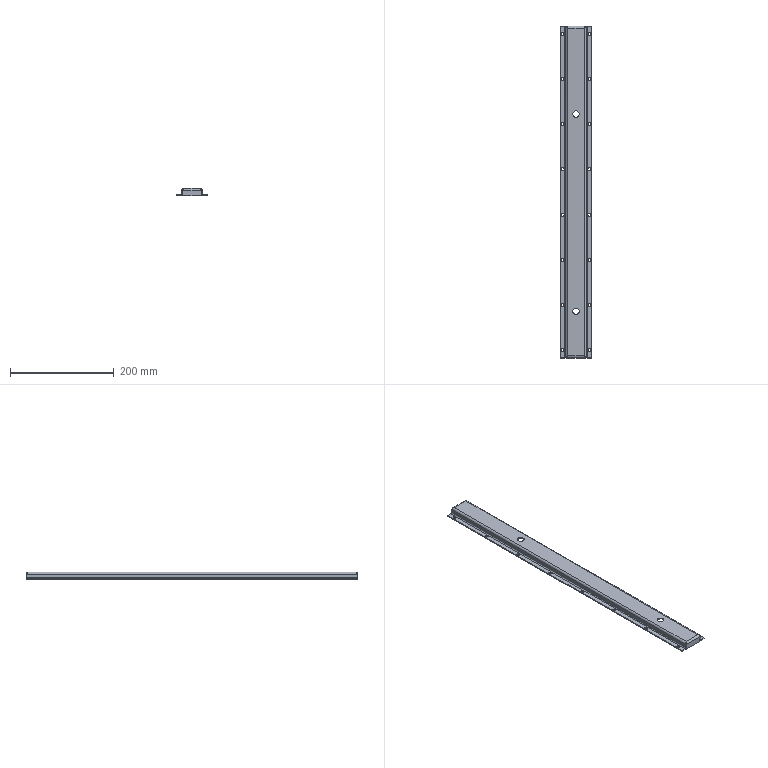Part | NX | features solid 2 | 1 solid | 110 faces | box 60 x 640 x 15 mm | volume 103697 mm3 | plane 50 | cylinder 48 | spline 12 | commonest cylinder face diameters 6 x32 4 x6 8 x6 12.6 x4